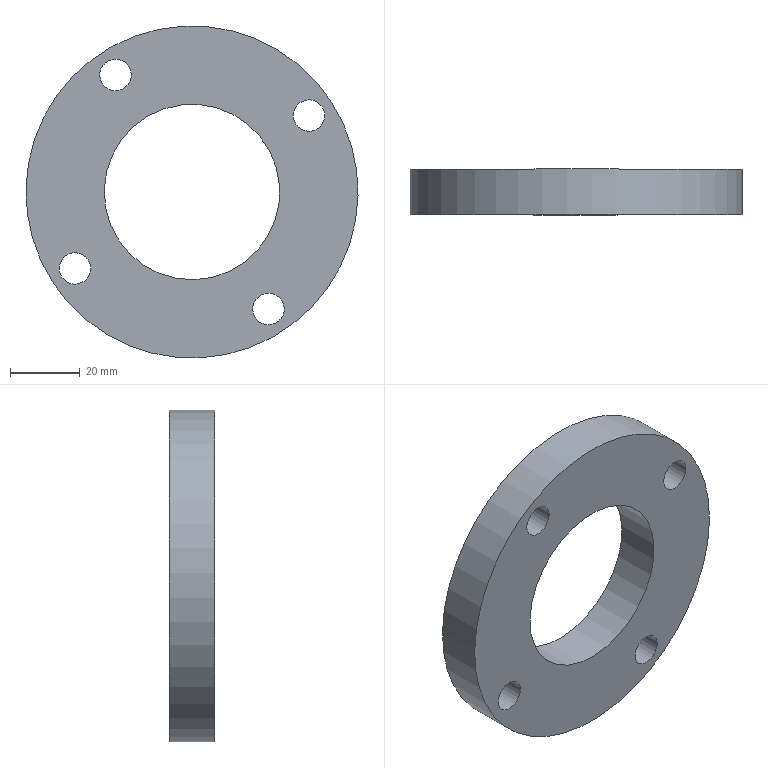Part | NX | features MAIN_BODY 2 | 1 solid | 8 faces | box 95 x 13 x 95 mm | volume 63109 mm3 | cylinder 6 | plane 2 | commonest cylinder face diameters 9 x4 50.2 x1 95 x1
STEP:
#1=CARTESIAN_POINT('',(29.72,994.,-192.583));
#2=VERTEX_POINT('',#1);
#3=CARTESIAN_POINT('',(33.487,994.,-190.122));
#4=DIRECTION('',(0.,1.,0.));
#5=DIRECTION('',(-0.8372,0.,-0.5469));
#6=AXIS2_PLACEMENT_3D('',#3,#4,#5);
#7=CIRCLE('',#6,4.5);
#8=EDGE_CURVE('',#2,#2,#7,.T.);
#9=ORIENTED_EDGE('',*,*,#8,.T.);
#10=EDGE_LOOP('',(#9));
#11=FACE_BOUND('',#10,.T.);
#12=CARTESIAN_POINT('',(29.72,981.,-192.583));
#13=VERTEX_POINT('',#12);
#14=CARTESIAN_POINT('',(33.487,981.,-190.122));
#15=DIRECTION('',(0.,1.,0.));
#16=DIRECTION('',(-0.8372,0.,-0.5469));
#17=AXIS2_PLACEMENT_3D('',#14,#15,#16);
#18=CIRCLE('',#17,4.5);
#19=EDGE_CURVE('',#13,#13,#18,.T.);
#20=ORIENTED_EDGE('',*,*,#19,.F.);
#21=EDGE_LOOP('',(#20));
#22=FACE_BOUND('',#21,.T.);
#23=CARTESIAN_POINT('',(33.487,994.,-190.122));
#24=DIRECTION('',(0.,-1.,0.));
#25=DIRECTION('',(0.8372,0.,0.5469));
#26=AXIS2_PLACEMENT_3D('',#23,#24,#25);
#27=CYLINDRICAL_SURFACE('',#26,4.5);
#28=ADVANCED_FACE('',(#11,#22),#27,.F.);
#29=CARTESIAN_POINT('',(-25.645,994.,-180.974));
#30=VERTEX_POINT('',#29);
#31=CARTESIAN_POINT('',(-21.878,994.,-178.513));
#32=DIRECTION('',(0.,1.,0.));
#33=DIRECTION('',(-0.8372,0.,-0.5469));
#34=AXIS2_PLACEMENT_3D('',#31,#32,#33);
#35=CIRCLE('',#34,4.5);
#36=EDGE_CURVE('',#30,#30,#35,.T.);
#37=ORIENTED_EDGE('',*,*,#36,.T.);
#38=EDGE_LOOP('',(#37));
#39=FACE_BOUND('',#38,.T.);
#40=CARTESIAN_POINT('',(-25.645,981.,-180.974));
#41=VERTEX_POINT('',#40);
#42=CARTESIAN_POINT('',(-21.878,981.,-178.513));
#43=DIRECTION('',(0.,1.,0.));
#44=DIRECTION('',(-0.8372,0.,-0.5469));
#45=AXIS2_PLACEMENT_3D('',#42,#43,#44);
#46=CIRCLE('',#45,4.5);
#47=EDGE_CURVE('',#41,#41,#46,.T.);
#48=ORIENTED_EDGE('',*,*,#47,.F.);
#49=EDGE_LOOP('',(#48));
#50=FACE_BOUND('',#49,.T.);
#51=CARTESIAN_POINT('',(-21.878,994.,-178.513));
#52=DIRECTION('',(0.,-1.,0.));
#53=DIRECTION('',(0.8372,0.,0.5469));
#54=AXIS2_PLACEMENT_3D('',#51,#52,#53);
#55=CYLINDRICAL_SURFACE('',#54,4.5);
#56=ADVANCED_FACE('',(#39,#50),#55,.F.);
#57=CARTESIAN_POINT('',(-37.254,994.,-236.339));
#58=VERTEX_POINT('',#57);
#59=CARTESIAN_POINT('',(-33.487,994.,-233.878));
#60=DIRECTION('',(0.,1.,0.));
#61=DIRECTION('',(-0.8372,0.,-0.5469));
#62=AXIS2_PLACEMENT_3D('',#59,#60,#61);
#63=CIRCLE('',#62,4.5);
#64=EDGE_CURVE('',#58,#58,#63,.T.);
#65=ORIENTED_EDGE('',*,*,#64,.T.);
#66=EDGE_LOOP('',(#65));
#67=FACE_BOUND('',#66,.T.);
#68=CARTESIAN_POINT('',(-37.254,981.,-236.339));
#69=VERTEX_POINT('',#68);
#70=CARTESIAN_POINT('',(-33.487,981.,-233.878));
#71=DIRECTION('',(0.,1.,0.));
#72=DIRECTION('',(-0.8372,0.,-0.5469));
#73=AXIS2_PLACEMENT_3D('',#70,#71,#72);
#74=CIRCLE('',#73,4.5);
#75=EDGE_CURVE('',#69,#69,#74,.T.);
#76=ORIENTED_EDGE('',*,*,#75,.F.);
#77=EDGE_LOOP('',(#76));
#78=FACE_BOUND('',#77,.T.);
#79=CARTESIAN_POINT('',(-33.487,994.,-233.878));
#80=DIRECTION('',(0.,-1.,0.));
#81=DIRECTION('',(0.8372,0.,0.5469));
#82=AXIS2_PLACEMENT_3D('',#79,#80,#81);
#83=CYLINDRICAL_SURFACE('',#82,4.5);
#84=ADVANCED_FACE('',(#67,#78),#83,.F.);
#85=CARTESIAN_POINT('',(18.111,994.,-247.948));
#86=VERTEX_POINT('',#85);
#87=CARTESIAN_POINT('',(21.878,994.,-245.487));
#88=DIRECTION('',(0.,1.,0.));
#89=DIRECTION('',(-0.8372,0.,-0.5469));
#90=AXIS2_PLACEMENT_3D('',#87,#88,#89);
#91=CIRCLE('',#90,4.5);
#92=EDGE_CURVE('',#86,#86,#91,.T.);
#93=ORIENTED_EDGE('',*,*,#92,.T.);
#94=EDGE_LOOP('',(#93));
#95=FACE_BOUND('',#94,.T.);
#96=CARTESIAN_POINT('',(18.111,981.,-247.948));
#97=VERTEX_POINT('',#96);
#98=CARTESIAN_POINT('',(21.878,981.,-245.487));
#99=DIRECTION('',(0.,1.,0.));
#100=DIRECTION('',(-0.8372,0.,-0.5469));
#101=AXIS2_PLACEMENT_3D('',#98,#99,#100);
#102=CIRCLE('',#101,4.5);
#103=EDGE_CURVE('',#97,#97,#102,.T.);
#104=ORIENTED_EDGE('',*,*,#103,.F.);
#105=EDGE_LOOP('',(#104));
#106=FACE_BOUND('',#105,.T.);
#107=CARTESIAN_POINT('',(21.878,994.,-245.487));
#108=DIRECTION('',(0.,-1.,0.));
#109=DIRECTION('',(0.8372,0.,0.5469));
#110=AXIS2_PLACEMENT_3D('',#107,#108,#109);
#111=CYLINDRICAL_SURFACE('',#110,4.5);
#112=ADVANCED_FACE('',(#95,#106),#111,.F.);
#113=CARTESIAN_POINT('',(-21.013,994.,-225.728));
#114=VERTEX_POINT('',#113);
#115=CARTESIAN_POINT('',(0.,994.,-212.));
#116=DIRECTION('',(0.,1.,0.));
#117=DIRECTION('',(-0.8372,0.,-0.5469));
#118=AXIS2_PLACEMENT_3D('',#115,#116,#117);
#119=CIRCLE('',#118,25.1);
#120=EDGE_CURVE('',#114,#114,#119,.T.);
#121=ORIENTED_EDGE('',*,*,#120,.T.);
#122=EDGE_LOOP('',(#121));
#123=FACE_BOUND('',#122,.T.);
#124=CARTESIAN_POINT('',(-21.013,981.,-225.728));
#125=VERTEX_POINT('',#124);
#126=CARTESIAN_POINT('',(0.,981.,-212.));
#127=DIRECTION('',(0.,1.,0.));
#128=DIRECTION('',(-0.8372,0.,-0.5469));
#129=AXIS2_PLACEMENT_3D('',#126,#127,#128);
#130=CIRCLE('',#129,25.1);
#131=EDGE_CURVE('',#125,#125,#130,.T.);
#132=ORIENTED_EDGE('',*,*,#131,.F.);
#133=EDGE_LOOP('',(#132));
#134=FACE_BOUND('',#133,.T.);
#135=CARTESIAN_POINT('',(0.,994.,-212.));
#136=DIRECTION('',(0.,-1.,0.));
#137=DIRECTION('',(0.8372,0.,0.5469));
#138=AXIS2_PLACEMENT_3D('',#135,#136,#137);
#139=CYLINDRICAL_SURFACE('',#138,25.1);
#140=ADVANCED_FACE('',(#123,#134),#139,.F.);
#141=CARTESIAN_POINT('',(-39.766,994.,-237.98));
#142=VERTEX_POINT('',#141);
#143=CARTESIAN_POINT('',(0.,994.,-212.));
#144=DIRECTION('',(0.,1.,0.));
#145=DIRECTION('',(-0.8372,0.,-0.5469));
#146=AXIS2_PLACEMENT_3D('',#143,#144,#145);
#147=CIRCLE('',#146,47.5);
#148=EDGE_CURVE('',#142,#142,#147,.T.);
#149=ORIENTED_EDGE('',*,*,#148,.F.);
#150=EDGE_LOOP('',(#149));
#151=FACE_BOUND('',#150,.T.);
#152=CARTESIAN_POINT('',(-39.766,981.,-237.98));
#153=VERTEX_POINT('',#152);
#154=CARTESIAN_POINT('',(0.,981.,-212.));
#155=DIRECTION('',(0.,1.,0.));
#156=DIRECTION('',(-0.8372,0.,-0.5469));
#157=AXIS2_PLACEMENT_3D('',#154,#155,#156);
#158=CIRCLE('',#157,47.5);
#159=EDGE_CURVE('',#153,#153,#158,.T.);
#160=ORIENTED_EDGE('',*,*,#159,.T.);
#161=EDGE_LOOP('',(#160));
#162=FACE_BOUND('',#161,.T.);
#163=CARTESIAN_POINT('',(0.,994.,-212.));
#164=DIRECTION('',(0.,-1.,0.));
#165=DIRECTION('',(0.8372,0.,0.5469));
#166=AXIS2_PLACEMENT_3D('',#163,#164,#165);
#167=CYLINDRICAL_SURFACE('',#166,47.5);
#168=ADVANCED_FACE('',(#151,#162),#167,.T.);
#169=ORIENTED_EDGE('',*,*,#120,.F.);
#170=EDGE_LOOP('',(#169));
#171=FACE_BOUND('',#170,.T.);
#172=ORIENTED_EDGE('',*,*,#92,.F.);
#173=EDGE_LOOP('',(#172));
#174=FACE_BOUND('',#173,.T.);
#175=ORIENTED_EDGE('',*,*,#64,.F.);
#176=EDGE_LOOP('',(#175));
#177=FACE_BOUND('',#176,.T.);
#178=ORIENTED_EDGE('',*,*,#36,.F.);
#179=EDGE_LOOP('',(#178));
#180=FACE_BOUND('',#179,.T.);
#181=ORIENTED_EDGE('',*,*,#8,.F.);
#182=EDGE_LOOP('',(#181));
#183=FACE_BOUND('',#182,.T.);
#184=ORIENTED_EDGE('',*,*,#148,.T.);
#185=EDGE_LOOP('',(#184));
#186=FACE_BOUND('',#185,.T.);
#187=CARTESIAN_POINT('',(0.,994.,-212.));
#188=DIRECTION('',(0.,1.,0.));
#189=DIRECTION('',(-0.8372,0.,-0.5469));
#190=AXIS2_PLACEMENT_3D('',#187,#188,#189);
#191=PLANE('',#190);
#192=ADVANCED_FACE('',(#171,#174,#177,#180,#183,#186),#191,.T.);
#193=ORIENTED_EDGE('',*,*,#131,.T.);
#194=EDGE_LOOP('',(#193));
#195=FACE_BOUND('',#194,.T.);
#196=ORIENTED_EDGE('',*,*,#103,.T.);
#197=EDGE_LOOP('',(#196));
#198=FACE_BOUND('',#197,.T.);
#199=ORIENTED_EDGE('',*,*,#75,.T.);
#200=EDGE_LOOP('',(#199));
#201=FACE_BOUND('',#200,.T.);
#202=ORIENTED_EDGE('',*,*,#47,.T.);
#203=EDGE_LOOP('',(#202));
#204=FACE_BOUND('',#203,.T.);
#205=ORIENTED_EDGE('',*,*,#19,.T.);
#206=EDGE_LOOP('',(#205));
#207=FACE_BOUND('',#206,.T.);
#208=ORIENTED_EDGE('',*,*,#159,.F.);
#209=EDGE_LOOP('',(#208));
#210=FACE_BOUND('',#209,.T.);
#211=CARTESIAN_POINT('',(0.,981.,-212.));
#212=DIRECTION('',(0.,1.,0.));
#213=DIRECTION('',(-0.8372,0.,-0.5469));
#214=AXIS2_PLACEMENT_3D('',#211,#212,#213);
#215=PLANE('',#214);
#216=ADVANCED_FACE('',(#195,#198,#201,#204,#207,#210),#215,.F.);
#217=CLOSED_SHELL('',(#28,#56,#84,#112,#140,#168,#192,#216));
#218=MANIFOLD_SOLID_BREP('',#217);
#219=(LENGTH_UNIT()NAMED_UNIT(*)SI_UNIT(.MILLI.,.METRE.));
#220=UNCERTAINTY_MEASURE_WITH_UNIT(LENGTH_MEASURE(0.00001),#219,'','');
#221=(NAMED_UNIT(*)PLANE_ANGLE_UNIT()SI_UNIT($,.RADIAN.));
#222=(NAMED_UNIT(*)SI_UNIT($,.STERADIAN.)SOLID_ANGLE_UNIT());
#223=(GEOMETRIC_REPRESENTATION_CONTEXT(3)GLOBAL_UNCERTAINTY_ASSIGNED_CONTEXT((#220))GLOBAL_UNIT_ASSIGNED_CONTEXT((#219,#221,#222))REPRESENTATION_CONTEXT('',''));
#224=ADVANCED_BREP_SHAPE_REPRESENTATION('',(#218),#223);